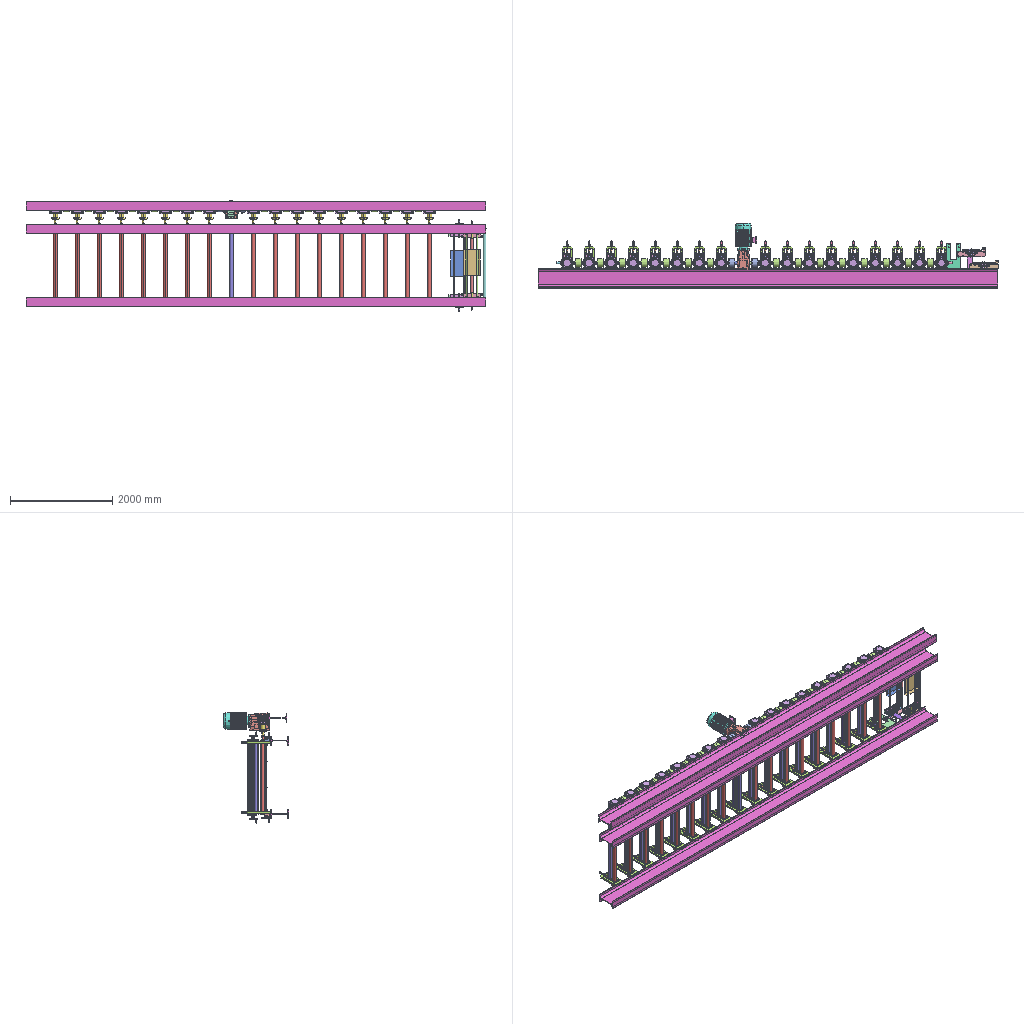Assembly | STEP file | 57 different items | 1331 placed | box 9007 x 1275 x 2167 mm
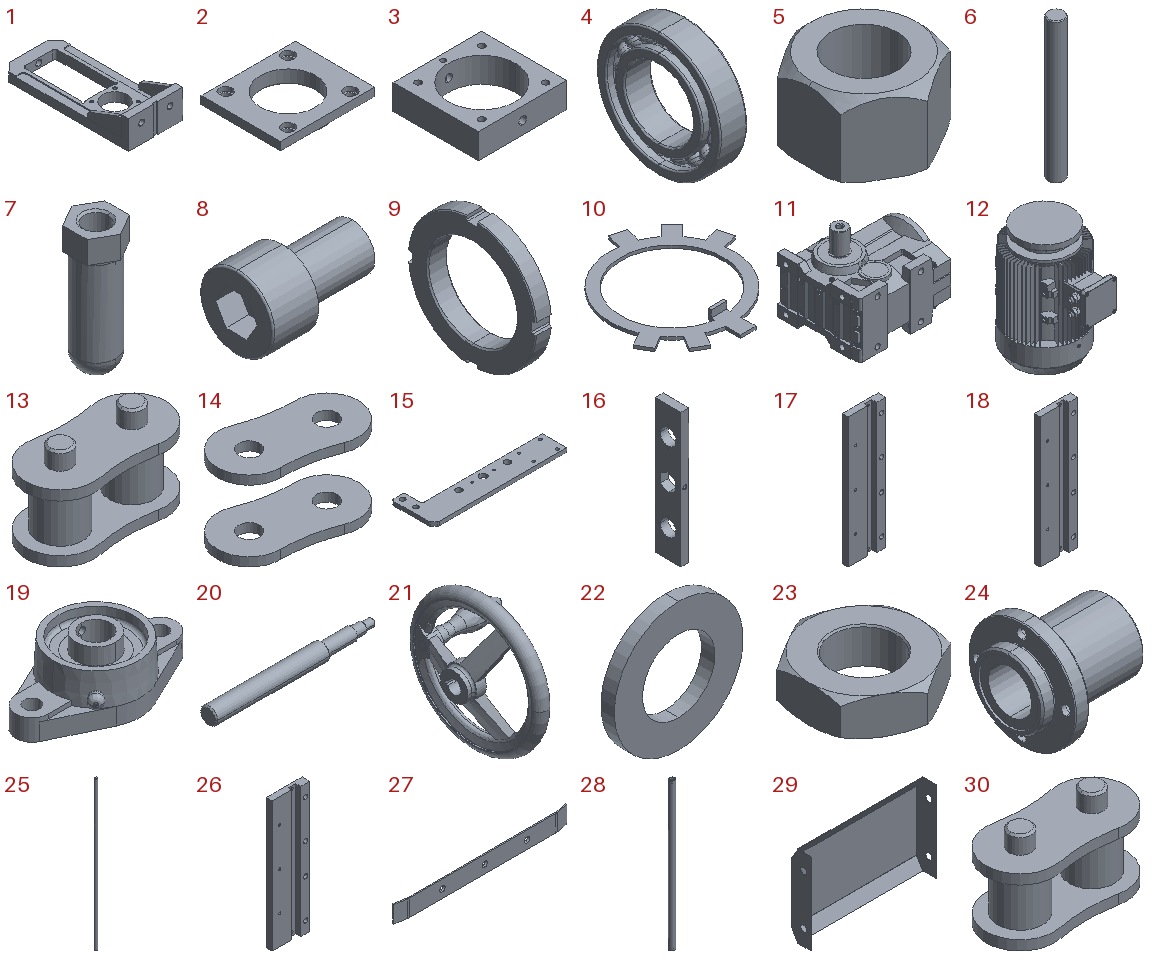Parts list (item | quantity | size | volume):
1 | x36 | 200 x 470 x 105 mm | 2366246 mm3
2 | x144 | 130 x 110 x 18 mm | 122243 mm3
3 | x36 | 120 x 115 x 34 mm | 242245 mm3
4 | x72 | 20 x 90 x 90 mm | 65276 mm3
5 | x72 | 28.536 x 32.95 x 19 mm | 8806 mm3
6 | x36 | 20 x 20 x 175 mm | 54917 mm3
7 | x36 | 30 x 34.641 x 92 mm | 50056 mm3
8 | x576 | 26 x 16 x 16 mm | 2981 mm3
9 | x72 | 11 x 69.742 x 69.742 mm | 20244 mm3
10 | x36 | 72.177 x 75.317 x 5 mm | 1971 mm3
11 | x1 | 389 x 345 x 416 mm | 22949319 mm3
12 | x1 | 323.2 x 423.482 x 518 mm | 31241978 mm3
13 | x17 | 37.13 x 18.08 x 26.9 mm | 6307 mm3
14 | x16 | 36.793 x 21.646 x 22.78 mm | 2638 mm3
15 | x2 | 549.959 x 175.002 x 16 mm | 892550 mm3
16 | x2 | 20 x 65 x 340 mm | 355958 mm3
17 | x1 | 92.98 x 19.5 x 340 mm | 429888 mm3
18 | x2 | 92.98 x 19.5 x 340 mm | 434524 mm3
19 | x2 | 113 x 62 x 37.3 mm | 69563 mm3
20 | x2 | 263 x 27 x 27 mm | 124305 mm3
21 | x2 | 117 x 160 x 160 mm | 172381 mm3
22 | x2 | 24 x 2.5 x 24 mm | 773.126 mm3
23 | x2 | 18 x 20.785 x 6 mm | 1162 mm3
24 | x4 | 59 x 62 x 62 mm | 56273 mm3
25 | x2 | 25 x 25 x 1510 mm | 741143 mm3
26 | x1 | 92.98 x 19.5 x 340 mm | 429888 mm3
27 | x4 | 409.088 x 8.069 x 40 mm | 48290 mm3
28 | x2 | 50 x 50 x 1450 mm | 1794980 mm3
29 | x1 | 504 x 80 x 327.138 mm | 217824 mm3
30 | x16 | 37.13 x 18.08 x 26.9 mm | 6307 mm3
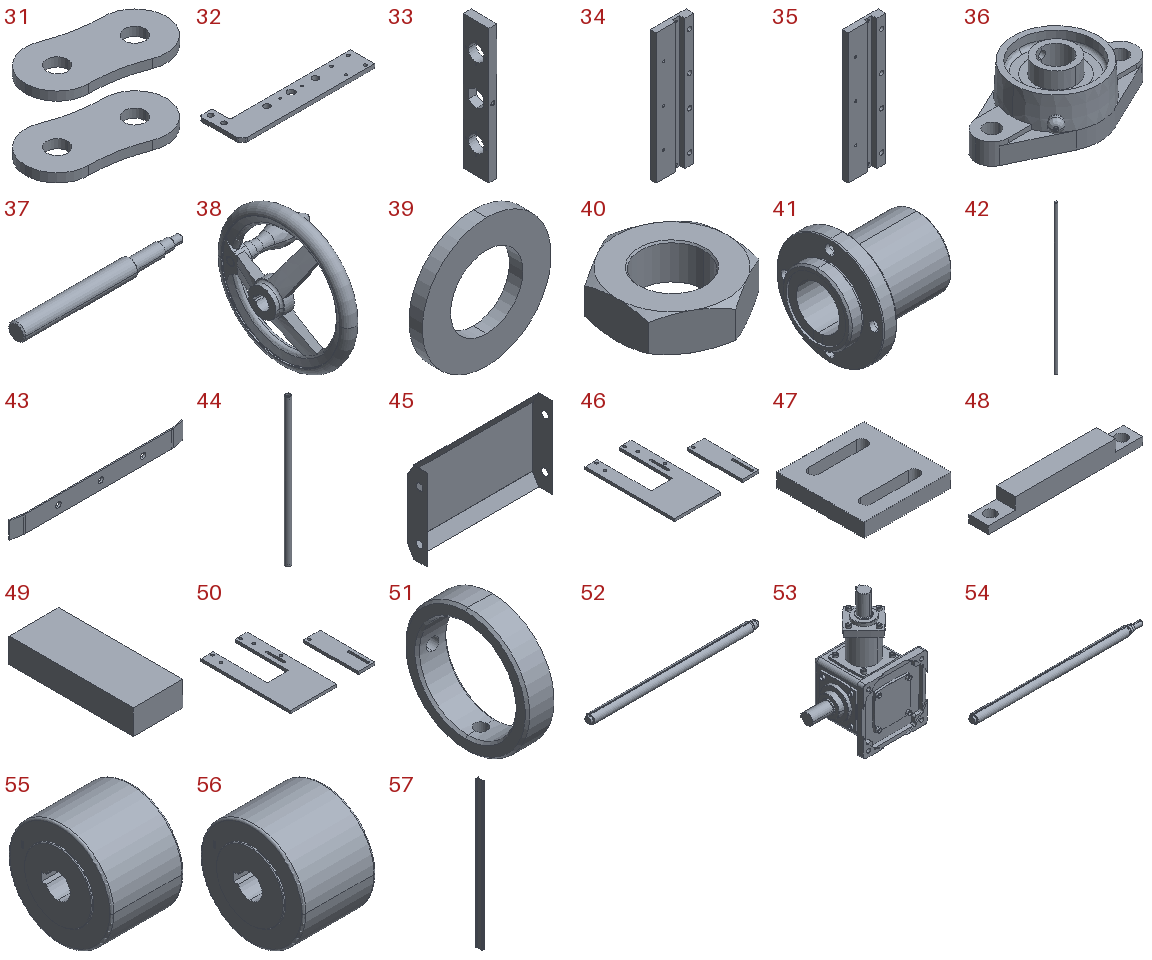31 | x16 | 36.793 x 21.646 x 22.78 mm | 2638 mm3
32 | x2 | 549.959 x 175.002 x 16 mm | 892550 mm3
33 | x2 | 20 x 65 x 340 mm | 355958 mm3
34 | x2 | 92.98 x 19.5 x 340 mm | 429888 mm3
35 | x2 | 92.98 x 19.5 x 340 mm | 434524 mm3
36 | x2 | 113 x 62 x 37.3 mm | 69563 mm3
37 | x2 | 263 x 27 x 27 mm | 124305 mm3
38 | x2 | 117 x 160 x 160 mm | 172381 mm3
39 | x2 | 24 x 2.5 x 24 mm | 773.126 mm3
40 | x2 | 18 x 20.785 x 6 mm | 1162 mm3
41 | x4 | 59 x 62 x 62 mm | 56273 mm3
42 | x2 | 25 x 25 x 1470 mm | 721508 mm3
43 | x4 | 409.088 x 8.069 x 40 mm | 48290 mm3
44 | x2 | 50 x 50 x 1410 mm | 1744715 mm3
45 | x1 | 504 x 80 x 327.138 mm | 217529 mm3
46 | x1 | 507 x 540 x 16 mm | 2169859 mm3
47 | x1 | 100 x 100 x 16 mm | 134073 mm3
48 | x1 | 200 x 25 x 25 mm | 95447 mm3
49 | x1 | 40 x 100 x 20 mm | 80000 mm3
50 | x1 | 507 x 540 x 16 mm | 2169859 mm3
51 | x8 | 8 x 32 x 32 mm | 2296 mm3
52 | x19 | 1430 x 75 x 75 mm | 6071398 mm3
53 | x17 | 416 x 229.5 x 425.5 mm | 8932434 mm3
54 | x17 | 1505 x 75 x 75 mm | 6161488 mm3
55 | x2 | 123.5 x 168 x 168 mm | 2239752 mm3
56 | x15 | 123.5 x 168 x 168 mm | 2326586 mm3
57 | x3 | 175 x 350 x 9000 mm | 85369066 mm3
Placements (level | parent | child | x y z in mm | rotation matrix by rows), first 402 of 1411 lines:
1 | subassembly 2 | subassembly 3 | 0.0 0.0 668.0 | 1 0 0 0 1 0 0 0 1
2 | subassembly 3 | subassembly 4 | -0.0 248.0 -0.0 | 1 0 0 0 1 0 0 0 1
2 | subassembly 3 | subassembly 5 | -0.0 150.0 34.0 | 1 0 0 0 1 0 0 0 1
2 | subassembly 3 | subassembly 5 | -0.0 280.0 34.0 | 1 0 0 0 1 0 0 0 1
2 | subassembly 3 | subassembly 5 | 0.0 280.0 0.0 | -1 0 0 0 1 0 0 0 -1
2 | subassembly 3 | subassembly 5 | 0.0 150.0 0.0 | -1 0 0 0 1 0 0 0 -1
2 | subassembly 3 | subassembly 6 | -0.0 282.5 -0.0 | 1 0 0 0 1 0 0 0 1
2 | subassembly 3 | subassembly 7 | -0.0 280.0 17.0 | 0 0 1 0 1 0 -1 0 0
2 | subassembly 3 | subassembly 7 | -0.0 150.0 17.0 | 0 0 1 0 1 0 -1 0 0
2 | subassembly 3 | subassembly 8 | -0.0 470.0 17.0 | 0.9291 0.3698 0 0 0 1 0.3698 -0.9291 0
2 | subassembly 3 | subassembly 8 | -0.0 411.0 17.0 | 1 0 0 0 0 1 0 -1 0
2 | subassembly 3 | subassembly 9 | -0.0 515.0 17.0 | -0.6523 0.7579 0 0 0 -1 -0.7579 -0.6523 -0
2 | subassembly 3 | subassembly 10 | -0.0 489.0 17.0 | 0.9291 -0.3698 0 0 0 -1 0.3698 0.9291 -0
2 | subassembly 3 | subassembly 11 | 42.999 107.001 -15.0 | 0 -0.4429 -0.8966 0 0.8966 -0.4429 1 0 0
2 | subassembly 3 | subassembly 11 | -42.999 107.001 -15.0 | 0 0.8966 -0.4429 0 0.4429 0.8966 1 0 0
2 | subassembly 3 | subassembly 11 | -42.999 237.001 49.0 | 0 -0.02998 -0.9996 0 -0.9996 0.02998 -1 0 0
2 | subassembly 3 | subassembly 11 | -42.999 322.999 49.0 | 0 -0.9996 0.02998 0 0.02998 0.9996 -1 0 0
2 | subassembly 3 | subassembly 11 | 42.999 192.999 -15.0 | 0 -0.8966 0.4429 0 -0.4429 -0.8966 1 0 0
2 | subassembly 3 | subassembly 11 | 42.999 237.001 -15.0 | 0 0.9996 0.02998 0 -0.02998 0.9996 1 0 0
2 | subassembly 3 | subassembly 11 | -42.999 192.999 -15.0 | 0 0.4429 0.8966 0 -0.8966 0.4429 1 0 0
2 | subassembly 3 | subassembly 11 | 42.999 237.001 49.0 | 0 0.9996 -0.02998 0 -0.02998 -0.9996 -1 0 0
2 | subassembly 3 | subassembly 11 | -42.999 192.999 49.0 | 0 0.4429 -0.8966 0 -0.8966 -0.4429 -1 0 0
2 | subassembly 3 | subassembly 11 | -42.999 322.999 -15.0 | 0 -0.9996 -0.02998 0 0.02998 -0.9996 1 0 0
2 | subassembly 3 | subassembly 11 | -42.999 107.001 49.0 | 0 0.8966 0.4429 0 0.4429 -0.8966 -1 0 0
2 | subassembly 3 | subassembly 11 | 42.999 107.001 49.0 | 0 -0.4429 0.8966 0 0.8966 0.4429 -1 0 0
2 | subassembly 3 | subassembly 11 | 42.999 322.999 49.0 | 0 0.02998 0.9996 0 0.9996 -0.02998 -1 0 0
2 | subassembly 3 | subassembly 11 | 42.999 192.999 49.0 | 0 -0.8966 -0.4429 0 -0.4429 0.8966 -1 0 0
2 | subassembly 3 | subassembly 11 | 42.999 322.999 -15.0 | 0 0.02998 -0.9996 0 0.9996 0.02998 1 0 0
2 | subassembly 3 | subassembly 11 | -42.999 237.001 -15.0 | 0 -0.02998 0.9996 0 -0.9996 -0.02998 1 0 0
1 | subassembly 2 | subassembly 12 | 431.0 -0.0 668.0 | 1 0 0 0 1 0 0 0 1
2 | subassembly 12 | subassembly 4 | -0.0 248.0 -0.0 | 1 0 0 0 1 0 0 0 1
2 | subassembly 12 | subassembly 5 | -0.0 280.0 34.0 | 1 0 0 0 1 0 0 0 1
2 | subassembly 12 | subassembly 5 | 0.0 280.0 0.0 | -1 0 0 0 1 0 0 0 -1
2 | subassembly 12 | subassembly 5 | 0.0 150.0 0.0 | -1 0 0 0 1 0 0 0 -1
2 | subassembly 12 | subassembly 5 | -0.0 150.0 34.0 | 1 0 0 0 1 0 0 0 1
2 | subassembly 12 | subassembly 6 | -0.0 282.5 -0.0 | 1 0 0 0 1 0 0 0 1
2 | subassembly 12 | subassembly 7 | -0.0 280.0 17.0 | 0 0 1 0 1 0 -1 0 0
2 | subassembly 12 | subassembly 7 | -0.0 150.0 17.0 | 0 0 1 0 1 0 -1 0 0
2 | subassembly 12 | subassembly 8 | -0.0 470.0 17.0 | 0.9291 0.3698 0 0 0 1 0.3698 -0.9291 0
2 | subassembly 12 | subassembly 8 | -0.0 411.0 17.0 | 1 0 0 0 0 1 0 -1 0
2 | subassembly 12 | subassembly 9 | -0.0 515.0 17.0 | -0.6523 0.7579 0 0 0 -1 -0.7579 -0.6523 -0
2 | subassembly 12 | subassembly 10 | -0.0 489.0 17.0 | 0.9291 -0.3698 0 0 0 -1 0.3698 0.9291 -0
2 | subassembly 12 | subassembly 11 | 42.999 237.001 49.0 | 0 0.9996 -0.02998 0 -0.02998 -0.9996 -1 0 0
2 | subassembly 12 | subassembly 11 | 42.999 322.999 49.0 | 0 0.02998 0.9996 0 0.9996 -0.02998 -1 0 0
2 | subassembly 12 | subassembly 11 | -42.999 237.001 49.0 | 0 -0.02998 -0.9996 0 -0.9996 0.02998 -1 0 0
2 | subassembly 12 | subassembly 11 | -42.999 192.999 49.0 | 0 0.4429 -0.8966 0 -0.8966 -0.4429 -1 0 0
2 | subassembly 12 | subassembly 11 | -42.999 322.999 49.0 | 0 -0.9996 0.02998 0 0.02998 0.9996 -1 0 0
2 | subassembly 12 | subassembly 11 | 42.999 107.001 49.0 | 0 -0.4429 0.8966 0 0.8966 0.4429 -1 0 0
2 | subassembly 12 | subassembly 11 | 42.999 192.999 -15.0 | 0 -0.8966 0.4429 0 -0.4429 -0.8966 1 0 0
2 | subassembly 12 | subassembly 11 | 42.999 237.001 -15.0 | 0 0.9996 0.02998 0 -0.02998 0.9996 1 0 0
2 | subassembly 12 | subassembly 11 | -42.999 237.001 -15.0 | 0 -0.02998 0.9996 0 -0.9996 -0.02998 1 0 0
2 | subassembly 12 | subassembly 11 | 42.999 192.999 49.0 | 0 -0.8966 -0.4429 0 -0.4429 0.8966 -1 0 0
2 | subassembly 12 | subassembly 11 | -42.999 107.001 -15.0 | 0 0.8966 -0.4429 0 0.4429 0.8966 1 0 0
2 | subassembly 12 | subassembly 11 | -42.999 107.001 49.0 | 0 0.8966 0.4429 0 0.4429 -0.8966 -1 0 0
2 | subassembly 12 | subassembly 11 | -42.999 322.999 -15.0 | 0 -0.9996 -0.02998 0 0.02998 -0.9996 1 0 0
2 | subassembly 12 | subassembly 11 | -42.999 192.999 -15.0 | 0 0.4429 0.8966 0 -0.8966 0.4429 1 0 0
2 | subassembly 12 | subassembly 11 | 42.999 107.001 -15.0 | 0 -0.4429 -0.8966 0 0.8966 -0.4429 1 0 0
2 | subassembly 12 | subassembly 11 | 42.999 322.999 -15.0 | 0 0.02998 -0.9996 0 0.9996 0.02998 1 0 0
1 | subassembly 2 | subassembly 13 | 862.0 -0.0 668.0 | 1 0 0 0 1 0 0 0 1
2 | subassembly 13 | subassembly 4 | -0.0 248.0 -0.0 | 1 0 0 0 1 0 0 0 1
2 | subassembly 13 | subassembly 5 | 0.0 280.0 0.0 | -1 0 0 0 1 0 0 0 -1
2 | subassembly 13 | subassembly 5 | -0.0 280.0 34.0 | 1 0 0 0 1 0 0 0 1
2 | subassembly 13 | subassembly 5 | -0.0 150.0 34.0 | 1 0 0 0 1 0 0 0 1
2 | subassembly 13 | subassembly 5 | 0.0 150.0 0.0 | -1 0 0 0 1 0 0 0 -1
2 | subassembly 13 | subassembly 6 | -0.0 282.5 -0.0 | 1 0 0 0 1 0 0 0 1
2 | subassembly 13 | subassembly 7 | -0.0 280.0 17.0 | 0 0 1 0 1 0 -1 0 0
2 | subassembly 13 | subassembly 7 | -0.0 150.0 17.0 | 0 0 1 0 1 0 -1 0 0
2 | subassembly 13 | subassembly 8 | -0.0 411.0 17.0 | 1 0 0 0 0 1 0 -1 0
2 | subassembly 13 | subassembly 8 | -0.0 470.0 17.0 | 0.9291 0.3698 0 0 0 1 0.3698 -0.9291 0
2 | subassembly 13 | subassembly 9 | -0.0 515.0 17.0 | -0.6523 0.7579 0 0 0 -1 -0.7579 -0.6523 -0
2 | subassembly 13 | subassembly 10 | -0.0 489.0 17.0 | 0.9291 -0.3698 0 0 0 -1 0.3698 0.9291 -0
2 | subassembly 13 | subassembly 11 | -42.999 237.001 49.0 | 0 -0.02998 -0.9996 0 -0.9996 0.02998 -1 0 0
2 | subassembly 13 | subassembly 11 | 42.999 322.999 49.0 | 0 0.02998 0.9996 0 0.9996 -0.02998 -1 0 0
2 | subassembly 13 | subassembly 11 | -42.999 107.001 49.0 | 0 0.8966 0.4429 0 0.4429 -0.8966 -1 0 0
2 | subassembly 13 | subassembly 11 | -42.999 322.999 -15.0 | 0 -0.9996 -0.02998 0 0.02998 -0.9996 1 0 0
2 | subassembly 13 | subassembly 11 | 42.999 237.001 49.0 | 0 0.9996 -0.02998 0 -0.02998 -0.9996 -1 0 0
2 | subassembly 13 | subassembly 11 | 42.999 322.999 -15.0 | 0 0.02998 -0.9996 0 0.9996 0.02998 1 0 0
2 | subassembly 13 | subassembly 11 | -42.999 192.999 -15.0 | 0 0.4429 0.8966 0 -0.8966 0.4429 1 0 0
2 | subassembly 13 | subassembly 11 | -42.999 237.001 -15.0 | 0 -0.02998 0.9996 0 -0.9996 -0.02998 1 0 0
2 | subassembly 13 | subassembly 11 | -42.999 322.999 49.0 | 0 -0.9996 0.02998 0 0.02998 0.9996 -1 0 0
2 | subassembly 13 | subassembly 11 | -42.999 192.999 49.0 | 0 0.4429 -0.8966 0 -0.8966 -0.4429 -1 0 0
2 | subassembly 13 | subassembly 11 | 42.999 107.001 49.0 | 0 -0.4429 0.8966 0 0.8966 0.4429 -1 0 0
2 | subassembly 13 | subassembly 11 | 42.999 192.999 49.0 | 0 -0.8966 -0.4429 0 -0.4429 0.8966 -1 0 0
2 | subassembly 13 | subassembly 11 | 42.999 237.001 -15.0 | 0 0.9996 0.02998 0 -0.02998 0.9996 1 0 0
2 | subassembly 13 | subassembly 11 | 42.999 107.001 -15.0 | 0 -0.4429 -0.8966 0 0.8966 -0.4429 1 0 0
2 | subassembly 13 | subassembly 11 | -42.999 107.001 -15.0 | 0 0.8966 -0.4429 0 0.4429 0.8966 1 0 0
2 | subassembly 13 | subassembly 11 | 42.999 192.999 -15.0 | 0 -0.8966 0.4429 0 -0.4429 -0.8966 1 0 0
1 | subassembly 2 | subassembly 14 | 1293.0 -0.0 668.0 | 1 0 0 0 1 0 0 0 1
2 | subassembly 14 | subassembly 4 | -0.0 248.0 -0.0 | 1 0 0 0 1 0 0 0 1
2 | subassembly 14 | subassembly 5 | -0.0 280.0 0.0 | -1 0 0 0 1 0 0 0 -1
2 | subassembly 14 | subassembly 5 | 0.0 150.0 0.0 | -1 0 0 0 1 0 0 0 -1
2 | subassembly 14 | subassembly 5 | -0.0 150.0 34.0 | 1 0 0 0 1 0 0 0 1
2 | subassembly 14 | subassembly 5 | -0.0 280.0 34.0 | 1 0 0 0 1 0 0 0 1
2 | subassembly 14 | subassembly 6 | -0.0 282.5 -0.0 | 1 0 0 0 1 0 0 0 1
2 | subassembly 14 | subassembly 7 | -0.0 150.0 17.0 | 0 0 1 0 1 0 -1 0 0
2 | subassembly 14 | subassembly 7 | -0.0 280.0 17.0 | 0 0 1 0 1 0 -1 0 0
2 | subassembly 14 | subassembly 8 | -0.0 470.0 17.0 | 0.9291 0.3698 0 0 0 1 0.3698 -0.9291 0
2 | subassembly 14 | subassembly 8 | -0.0 411.0 17.0 | 1 0 0 0 0 1 0 -1 0
2 | subassembly 14 | subassembly 9 | 0.0 515.0 17.0 | -0.6523 0.7579 0 0 0 -1 -0.7579 -0.6523 -0
2 | subassembly 14 | subassembly 10 | 0.0 489.0 17.0 | 0.9291 -0.3698 0 0 0 -1 0.3698 0.9291 -0
2 | subassembly 14 | subassembly 11 | -42.999 192.999 49.0 | 0 0.4429 -0.8966 0 -0.8966 -0.4429 -1 0 0
2 | subassembly 14 | subassembly 11 | 42.999 237.001 -15.0 | 0 0.9996 0.02998 0 -0.02998 0.9996 1 0 0
2 | subassembly 14 | subassembly 11 | 42.999 322.999 49.0 | 0 0.02998 0.9996 0 0.9996 -0.02998 -1 0 0
2 | subassembly 14 | subassembly 11 | 42.999 107.001 -15.0 | 0 -0.4429 -0.8966 0 0.8966 -0.4429 1 0 0
2 | subassembly 14 | subassembly 11 | -42.999 107.001 49.0 | 0 0.8966 0.4429 0 0.4429 -0.8966 -1 0 0
2 | subassembly 14 | subassembly 11 | 42.999 322.999 -15.0 | 0 0.02998 -0.9996 0 0.9996 0.02998 1 0 0
2 | subassembly 14 | subassembly 11 | -42.999 322.999 -15.0 | 0 -0.9996 -0.02998 0 0.02998 -0.9996 1 0 0
2 | subassembly 14 | subassembly 11 | -42.999 192.999 -15.0 | 0 0.4429 0.8966 0 -0.8966 0.4429 1 0 0
2 | subassembly 14 | subassembly 11 | 42.999 237.001 49.0 | 0 0.9996 -0.02998 0 -0.02998 -0.9996 -1 0 0
2 | subassembly 14 | subassembly 11 | 42.999 192.999 49.0 | 0 -0.8966 -0.4429 0 -0.4429 0.8966 -1 0 0
2 | subassembly 14 | subassembly 11 | -42.999 237.001 -15.0 | 0 -0.02998 0.9996 0 -0.9996 -0.02998 1 0 0
2 | subassembly 14 | subassembly 11 | -42.999 237.001 49.0 | 0 -0.02998 -0.9996 0 -0.9996 0.02998 -1 0 0
2 | subassembly 14 | subassembly 11 | 42.999 107.001 49.0 | 0 -0.4429 0.8966 0 0.8966 0.4429 -1 0 0
2 | subassembly 14 | subassembly 11 | 42.999 192.999 -15.0 | 0 -0.8966 0.4429 0 -0.4429 -0.8966 1 0 0
2 | subassembly 14 | subassembly 11 | -42.999 107.001 -15.0 | 0 0.8966 -0.4429 0 0.4429 0.8966 1 0 0
2 | subassembly 14 | subassembly 11 | -42.999 322.999 49.0 | 0 -0.9996 0.02998 0 0.02998 0.9996 -1 0 0
1 | subassembly 2 | subassembly 15 | 1724.0 -0.0 668.0 | 1 0 0 0 1 0 0 0 1
2 | subassembly 15 | subassembly 4 | -0.0 248.0 -0.0 | 1 0 0 0 1 0 0 0 1
2 | subassembly 15 | subassembly 5 | -0.0 280.0 34.0 | 1 0 0 0 1 0 0 0 1
2 | subassembly 15 | subassembly 5 | 0.0 150.0 0.0 | -1 0 0 0 1 0 0 0 -1
2 | subassembly 15 | subassembly 5 | -0.0 280.0 0.0 | -1 0 0 0 1 0 0 0 -1
2 | subassembly 15 | subassembly 5 | -0.0 150.0 34.0 | 1 0 0 0 1 0 0 0 1
2 | subassembly 15 | subassembly 6 | -0.0 282.5 -0.0 | 1 0 0 0 1 0 0 0 1
2 | subassembly 15 | subassembly 7 | -0.0 280.0 17.0 | 0 0 1 0 1 0 -1 0 0
2 | subassembly 15 | subassembly 7 | -0.0 150.0 17.0 | 0 0 1 0 1 0 -1 0 0
2 | subassembly 15 | subassembly 8 | -0.0 470.0 17.0 | 0.9291 0.3698 0 0 0 1 0.3698 -0.9291 0
2 | subassembly 15 | subassembly 8 | -0.0 411.0 17.0 | 1 0 0 0 0 1 0 -1 0
2 | subassembly 15 | subassembly 9 | 0.0 515.0 17.0 | -0.6523 0.7579 0 0 0 -1 -0.7579 -0.6523 -0
2 | subassembly 15 | subassembly 10 | 0.0 489.0 17.0 | 0.9291 -0.3698 0 0 0 -1 0.3698 0.9291 -0
2 | subassembly 15 | subassembly 11 | 42.999 237.001 49.0 | 0 0.9996 -0.02998 0 -0.02998 -0.9996 -1 0 0
2 | subassembly 15 | subassembly 11 | 42.999 192.999 49.0 | 0 -0.8966 -0.4429 0 -0.4429 0.8966 -1 0 0
2 | subassembly 15 | subassembly 11 | 42.999 107.001 49.0 | 0 -0.4429 0.8966 0 0.8966 0.4429 -1 0 0
2 | subassembly 15 | subassembly 11 | 42.999 322.999 49.0 | 0 0.02998 0.9996 0 0.9996 -0.02998 -1 0 0
2 | subassembly 15 | subassembly 11 | 42.999 322.999 -15.0 | 0 0.02998 -0.9996 0 0.9996 0.02998 1 0 0
2 | subassembly 15 | subassembly 11 | 42.999 237.001 -15.0 | 0 0.9996 0.02998 0 -0.02998 0.9996 1 0 0
2 | subassembly 15 | subassembly 11 | 42.999 107.001 -15.0 | 0 -0.4429 -0.8966 0 0.8966 -0.4429 1 0 0
2 | subassembly 15 | subassembly 11 | -42.999 107.001 -15.0 | 0 0.8966 -0.4429 0 0.4429 0.8966 1 0 0
2 | subassembly 15 | subassembly 11 | -42.999 237.001 -15.0 | 0 -0.02998 0.9996 0 -0.9996 -0.02998 1 0 0
2 | subassembly 15 | subassembly 11 | -42.999 237.001 49.0 | 0 -0.02998 -0.9996 0 -0.9996 0.02998 -1 0 0
2 | subassembly 15 | subassembly 11 | 42.999 192.999 -15.0 | 0 -0.8966 0.4429 0 -0.4429 -0.8966 1 0 0
2 | subassembly 15 | subassembly 11 | -42.999 322.999 49.0 | 0 -0.9996 0.02998 0 0.02998 0.9996 -1 0 0
2 | subassembly 15 | subassembly 11 | -42.999 107.001 49.0 | 0 0.8966 0.4429 0 0.4429 -0.8966 -1 0 0
2 | subassembly 15 | subassembly 11 | -42.999 322.999 -15.0 | 0 -0.9996 -0.02998 0 0.02998 -0.9996 1 0 0
2 | subassembly 15 | subassembly 11 | -42.999 192.999 49.0 | 0 0.4429 -0.8966 0 -0.8966 -0.4429 -1 0 0
2 | subassembly 15 | subassembly 11 | -42.999 192.999 -15.0 | 0 0.4429 0.8966 0 -0.8966 0.4429 1 0 0
1 | subassembly 2 | subassembly 16 | 2155.0 -0.0 668.0 | 1 0 0 0 1 0 0 0 1
2 | subassembly 16 | subassembly 4 | -0.0 248.0 -0.0 | 1 0 0 0 1 0 0 0 1
2 | subassembly 16 | subassembly 5 | -0.0 150.0 34.0 | 1 0 0 0 1 0 0 0 1
2 | subassembly 16 | subassembly 5 | 0.0 150.0 0.0 | -1 0 0 0 1 0 0 0 -1
2 | subassembly 16 | subassembly 5 | -0.0 280.0 0.0 | -1 0 0 0 1 0 0 0 -1
2 | subassembly 16 | subassembly 5 | -0.0 280.0 34.0 | 1 0 0 0 1 0 0 0 1
2 | subassembly 16 | subassembly 6 | -0.0 282.5 -0.0 | 1 0 0 0 1 0 0 0 1
2 | subassembly 16 | subassembly 7 | -0.0 280.0 17.0 | 0 0 1 0 1 0 -1 0 0
2 | subassembly 16 | subassembly 7 | -0.0 150.0 17.0 | 0 0 1 0 1 0 -1 0 0
2 | subassembly 16 | subassembly 8 | -0.0 470.0 17.0 | 0.9291 0.3698 0 0 0 1 0.3698 -0.9291 0
2 | subassembly 16 | subassembly 8 | -0.0 411.0 17.0 | 1 0 0 0 0 1 0 -1 0
2 | subassembly 16 | subassembly 9 | 0.0 515.0 17.0 | -0.6523 0.7579 0 0 0 -1 -0.7579 -0.6523 -0
2 | subassembly 16 | subassembly 10 | 0.0 489.0 17.0 | 0.9291 -0.3698 0 0 0 -1 0.3698 0.9291 -0
2 | subassembly 16 | subassembly 11 | 42.999 237.001 -15.0 | 0 0.9996 0.02998 0 -0.02998 0.9996 1 0 0
2 | subassembly 16 | subassembly 11 | -42.999 237.001 -15.0 | 0 -0.02998 0.9996 0 -0.9996 -0.02998 1 0 0
2 | subassembly 16 | subassembly 11 | -42.999 237.001 49.0 | 0 -0.02998 -0.9996 0 -0.9996 0.02998 -1 0 0
2 | subassembly 16 | subassembly 11 | -42.999 192.999 49.0 | 0 0.4429 -0.8966 0 -0.8966 -0.4429 -1 0 0
2 | subassembly 16 | subassembly 11 | 42.999 192.999 49.0 | 0 -0.8966 -0.4429 0 -0.4429 0.8966 -1 0 0
2 | subassembly 16 | subassembly 11 | -42.999 192.999 -15.0 | 0 0.4429 0.8966 0 -0.8966 0.4429 1 0 0
2 | subassembly 16 | subassembly 11 | -42.999 107.001 49.0 | 0 0.8966 0.4429 0 0.4429 -0.8966 -1 0 0
2 | subassembly 16 | subassembly 11 | 42.999 107.001 49.0 | 0 -0.4429 0.8966 0 0.8966 0.4429 -1 0 0
2 | subassembly 16 | subassembly 11 | -42.999 107.001 -15.0 | 0 0.8966 -0.4429 0 0.4429 0.8966 1 0 0
2 | subassembly 16 | subassembly 11 | 42.999 107.001 -15.0 | 0 -0.4429 -0.8966 0 0.8966 -0.4429 1 0 0
2 | subassembly 16 | subassembly 11 | 42.999 192.999 -15.0 | 0 -0.8966 0.4429 0 -0.4429 -0.8966 1 0 0
2 | subassembly 16 | subassembly 11 | -42.999 322.999 49.0 | 0 -0.9996 0.02998 0 0.02998 0.9996 -1 0 0
2 | subassembly 16 | subassembly 11 | 42.999 237.001 49.0 | 0 0.9996 -0.02998 0 -0.02998 -0.9996 -1 0 0
2 | subassembly 16 | subassembly 11 | -42.999 322.999 -15.0 | 0 -0.9996 -0.02998 0 0.02998 -0.9996 1 0 0
2 | subassembly 16 | subassembly 11 | 42.999 322.999 49.0 | 0 0.02998 0.9996 0 0.9996 -0.02998 -1 0 0
2 | subassembly 16 | subassembly 11 | 42.999 322.999 -15.0 | 0 0.02998 -0.9996 0 0.9996 0.02998 1 0 0
1 | subassembly 2 | subassembly 17 | 2586.0 -0.0 668.0 | 1 0 0 0 1 0 0 0 1
2 | subassembly 17 | subassembly 4 | -0.0 248.0 -0.0 | 1 0 0 0 1 0 0 0 1
2 | subassembly 17 | subassembly 5 | -0.0 280.0 34.0 | 1 0 0 0 1 0 0 0 1
2 | subassembly 17 | subassembly 5 | -0.0 150.0 34.0 | 1 0 0 0 1 0 0 0 1
2 | subassembly 17 | subassembly 5 | -0.0 280.0 0.0 | -1 0 0 0 1 0 0 0 -1
2 | subassembly 17 | subassembly 5 | 0.0 150.0 0.0 | -1 0 0 0 1 0 0 0 -1
2 | subassembly 17 | subassembly 6 | -0.0 282.5 -0.0 | 1 0 0 0 1 0 0 0 1
2 | subassembly 17 | subassembly 7 | -0.0 150.0 17.0 | 0 0 1 0 1 0 -1 0 0
2 | subassembly 17 | subassembly 7 | -0.0 280.0 17.0 | 0 0 1 0 1 0 -1 0 0
2 | subassembly 17 | subassembly 8 | -0.0 411.0 17.0 | 1 0 0 0 0 1 0 -1 0
2 | subassembly 17 | subassembly 8 | -0.0 470.0 17.0 | 0.9291 0.3698 0 0 0 1 0.3698 -0.9291 0
2 | subassembly 17 | subassembly 9 | 0.0 515.0 17.0 | -0.6523 0.7579 0 0 0 -1 -0.7579 -0.6523 -0
2 | subassembly 17 | subassembly 10 | 0.0 489.0 17.0 | 0.9291 -0.3698 0 0 0 -1 0.3698 0.9291 -0
2 | subassembly 17 | subassembly 11 | 42.999 107.001 49.0 | 0 -0.4429 0.8966 0 0.8966 0.4429 -1 0 0
2 | subassembly 17 | subassembly 11 | -42.999 237.001 49.0 | 0 -0.02998 -0.9996 0 -0.9996 0.02998 -1 0 0
2 | subassembly 17 | subassembly 11 | 42.999 237.001 49.0 | 0 0.9996 -0.02998 0 -0.02998 -0.9996 -1 0 0
2 | subassembly 17 | subassembly 11 | -42.999 237.001 -15.0 | 0 -0.02998 0.9996 0 -0.9996 -0.02998 1 0 0
2 | subassembly 17 | subassembly 11 | -42.999 107.001 -15.0 | 0 0.8966 -0.4429 0 0.4429 0.8966 1 0 0
2 | subassembly 17 | subassembly 11 | -42.999 322.999 -15.0 | 0 -0.9996 -0.02998 0 0.02998 -0.9996 1 0 0
2 | subassembly 17 | subassembly 11 | -42.999 192.999 49.0 | 0 0.4429 -0.8966 0 -0.8966 -0.4429 -1 0 0
2 | subassembly 17 | subassembly 11 | 42.999 192.999 -15.0 | 0 -0.8966 0.4429 0 -0.4429 -0.8966 1 0 0
2 | subassembly 17 | subassembly 11 | -42.999 322.999 49.0 | 0 -0.9996 0.02998 0 0.02998 0.9996 -1 0 0
2 | subassembly 17 | subassembly 11 | 42.999 192.999 49.0 | 0 -0.8966 -0.4429 0 -0.4429 0.8966 -1 0 0
2 | subassembly 17 | subassembly 11 | 42.999 237.001 -15.0 | 0 0.9996 0.02998 0 -0.02998 0.9996 1 0 0
2 | subassembly 17 | subassembly 11 | 42.999 322.999 -15.0 | 0 0.02998 -0.9996 0 0.9996 0.02998 1 0 0
2 | subassembly 17 | subassembly 11 | -42.999 192.999 -15.0 | 0 0.4429 0.8966 0 -0.8966 0.4429 1 0 0
2 | subassembly 17 | subassembly 11 | -42.999 107.001 49.0 | 0 0.8966 0.4429 0 0.4429 -0.8966 -1 0 0
2 | subassembly 17 | subassembly 11 | 42.999 107.001 -15.0 | 0 -0.4429 -0.8966 0 0.8966 -0.4429 1 0 0
2 | subassembly 17 | subassembly 11 | 42.999 322.999 49.0 | 0 0.02998 0.9996 0 0.9996 -0.02998 -1 0 0
1 | subassembly 2 | subassembly 18 | 3017.0 -0.0 668.0 | 1 0 0 0 1 0 0 0 1
2 | subassembly 18 | subassembly 4 | -0.0 248.0 -0.0 | 1 0 0 0 1 0 0 0 1
2 | subassembly 18 | subassembly 5 | -0.0 280.0 34.0 | 1 0 0 0 1 0 0 0 1
2 | subassembly 18 | subassembly 5 | -0.0 150.0 34.0 | 1 0 0 0 1 0 0 0 1
2 | subassembly 18 | subassembly 5 | -0.0 280.0 0.0 | -1 0 0 0 1 0 0 0 -1
2 | subassembly 18 | subassembly 5 | 0.0 150.0 0.0 | -1 0 0 0 1 0 0 0 -1
2 | subassembly 18 | subassembly 6 | -0.0 282.5 -0.0 | 1 0 0 0 1 0 0 0 1
2 | subassembly 18 | subassembly 7 | -0.0 150.0 17.0 | 0 0 1 0 1 0 -1 0 0
2 | subassembly 18 | subassembly 7 | -0.0 280.0 17.0 | 0 0 1 0 1 0 -1 0 0
2 | subassembly 18 | subassembly 8 | -0.0 411.0 17.0 | 1 0 0 0 0 1 0 -1 0
2 | subassembly 18 | subassembly 8 | -0.0 470.0 17.0 | 0.9291 0.3698 0 0 0 1 0.3698 -0.9291 0
2 | subassembly 18 | subassembly 9 | 0.0 515.0 17.0 | -0.6523 0.7579 0 0 0 -1 -0.7579 -0.6523 -0
2 | subassembly 18 | subassembly 10 | 0.0 489.0 17.0 | 0.9291 -0.3698 0 0 0 -1 0.3698 0.9291 -0
2 | subassembly 18 | subassembly 11 | -42.999 192.999 49.0 | 0 0.4429 -0.8966 0 -0.8966 -0.4429 -1 0 0
2 | subassembly 18 | subassembly 11 | -42.999 192.999 -15.0 | 0 0.4429 0.8966 0 -0.8966 0.4429 1 0 0
2 | subassembly 18 | subassembly 11 | 42.999 107.001 -15.0 | 0 -0.4429 -0.8966 0 0.8966 -0.4429 1 0 0
2 | subassembly 18 | subassembly 11 | 42.999 237.001 49.0 | 0 0.9996 -0.02998 0 -0.02998 -0.9996 -1 0 0
2 | subassembly 18 | subassembly 11 | -42.999 322.999 49.0 | 0 -0.9996 0.02998 0 0.02998 0.9996 -1 0 0
2 | subassembly 18 | subassembly 11 | -42.999 107.001 -15.0 | 0 0.8966 -0.4429 0 0.4429 0.8966 1 0 0
2 | subassembly 18 | subassembly 11 | 42.999 322.999 49.0 | 0 0.02998 0.9996 0 0.9996 -0.02998 -1 0 0
2 | subassembly 18 | subassembly 11 | -42.999 107.001 49.0 | 0 0.8966 0.4429 0 0.4429 -0.8966 -1 0 0
2 | subassembly 18 | subassembly 11 | -42.999 322.999 -15.0 | 0 -0.9996 -0.02998 0 0.02998 -0.9996 1 0 0
2 | subassembly 18 | subassembly 11 | 42.999 107.001 49.0 | 0 -0.4429 0.8966 0 0.8966 0.4429 -1 0 0
2 | subassembly 18 | subassembly 11 | 42.999 192.999 -15.0 | 0 -0.8966 0.4429 0 -0.4429 -0.8966 1 0 0
2 | subassembly 18 | subassembly 11 | 42.999 322.999 -15.0 | 0 0.02998 -0.9996 0 0.9996 0.02998 1 0 0
2 | subassembly 18 | subassembly 11 | 42.999 237.001 -15.0 | 0 0.9996 0.02998 0 -0.02998 0.9996 1 0 0
2 | subassembly 18 | subassembly 11 | -42.999 237.001 -15.0 | 0 -0.02998 0.9996 0 -0.9996 -0.02998 1 0 0
2 | subassembly 18 | subassembly 11 | 42.999 192.999 49.0 | 0 -0.8966 -0.4429 0 -0.4429 0.8966 -1 0 0
2 | subassembly 18 | subassembly 11 | -42.999 237.001 49.0 | 0 -0.02998 -0.9996 0 -0.9996 0.02998 -1 0 0
1 | subassembly 2 | subassembly 19 | 3448.0 -0.0 668.0 | 1 0 0 0 1 0 0 0 1
2 | subassembly 19 | subassembly 4 | -0.0 248.0 -0.0 | 1 0 0 0 1 0 0 0 1
2 | subassembly 19 | subassembly 5 | -0.0 280.0 34.0 | 1 0 0 0 1 0 0 0 1
2 | subassembly 19 | subassembly 5 | 0.0 150.0 0.0 | -1 0 0 0 1 0 0 0 -1
2 | subassembly 19 | subassembly 5 | -0.0 150.0 34.0 | 1 0 0 0 1 0 0 0 1
2 | subassembly 19 | subassembly 5 | -0.0 280.0 0.0 | -1 0 0 0 1 0 0 0 -1
2 | subassembly 19 | subassembly 6 | -0.0 282.5 -0.0 | 1 0 0 0 1 0 0 0 1
2 | subassembly 19 | subassembly 7 | -0.0 280.0 17.0 | 0 0 1 0 1 0 -1 0 0
2 | subassembly 19 | subassembly 7 | -0.0 150.0 17.0 | 0 0 1 0 1 0 -1 0 0
2 | subassembly 19 | subassembly 8 | -0.0 411.0 17.0 | 1 0 0 0 0 1 0 -1 0
2 | subassembly 19 | subassembly 8 | -0.0 470.0 17.0 | 0.9291 0.3698 0 0 0 1 0.3698 -0.9291 0
2 | subassembly 19 | subassembly 9 | 0.0 515.0 17.0 | -0.6523 0.7579 0 0 0 -1 -0.7579 -0.6523 -0
2 | subassembly 19 | subassembly 10 | 0.0 489.0 17.0 | 0.9291 -0.3698 0 0 0 -1 0.3698 0.9291 -0
2 | subassembly 19 | subassembly 11 | -42.999 107.001 49.0 | 0 0.8966 0.4429 0 0.4429 -0.8966 -1 0 0
2 | subassembly 19 | subassembly 11 | 42.999 107.001 49.0 | 0 -0.4429 0.8966 0 0.8966 0.4429 -1 0 0
2 | subassembly 19 | subassembly 11 | -42.999 237.001 -15.0 | 0 -0.02998 0.9996 0 -0.9996 -0.02998 1 0 0
2 | subassembly 19 | subassembly 11 | -42.999 192.999 -15.0 | 0 0.4429 0.8966 0 -0.8966 0.4429 1 0 0
2 | subassembly 19 | subassembly 11 | -42.999 192.999 49.0 | 0 0.4429 -0.8966 0 -0.8966 -0.4429 -1 0 0
2 | subassembly 19 | subassembly 11 | -42.999 107.001 -15.0 | 0 0.8966 -0.4429 0 0.4429 0.8966 1 0 0
2 | subassembly 19 | subassembly 11 | -42.999 237.001 49.0 | 0 -0.02998 -0.9996 0 -0.9996 0.02998 -1 0 0
2 | subassembly 19 | subassembly 11 | 42.999 237.001 49.0 | 0 0.9996 -0.02998 0 -0.02998 -0.9996 -1 0 0
2 | subassembly 19 | subassembly 11 | -42.999 322.999 -15.0 | 0 -0.9996 -0.02998 0 0.02998 -0.9996 1 0 0
2 | subassembly 19 | subassembly 11 | 42.999 322.999 49.0 | 0 0.02998 0.9996 0 0.9996 -0.02998 -1 0 0
2 | subassembly 19 | subassembly 11 | 42.999 237.001 -15.0 | 0 0.9996 0.02998 0 -0.02998 0.9996 1 0 0
2 | subassembly 19 | subassembly 11 | 42.999 192.999 -15.0 | 0 -0.8966 0.4429 0 -0.4429 -0.8966 1 0 0
2 | subassembly 19 | subassembly 11 | 42.999 192.999 49.0 | 0 -0.8966 -0.4429 0 -0.4429 0.8966 -1 0 0
2 | subassembly 19 | subassembly 11 | 42.999 322.999 -15.0 | 0 0.02998 -0.9996 0 0.9996 0.02998 1 0 0
2 | subassembly 19 | subassembly 11 | -42.999 322.999 49.0 | 0 -0.9996 0.02998 0 0.02998 0.9996 -1 0 0
2 | subassembly 19 | subassembly 11 | 42.999 107.001 -15.0 | 0 -0.4429 -0.8966 0 0.8966 -0.4429 1 0 0
1 | subassembly 2 | subassembly 20 | 3879.0 0.0 668.0 | 1 0 0 0 1 0 0 0 1
2 | subassembly 20 | subassembly 4 | -0.0 248.0 -0.0 | 1 0 0 0 1 0 0 0 1
2 | subassembly 20 | subassembly 5 | -0.0 280.0 34.0 | 1 0 0 0 1 0 0 0 1
2 | subassembly 20 | subassembly 5 | 0.0 150.0 0.0 | -1 0 0 0 1 0 0 0 -1
2 | subassembly 20 | subassembly 5 | -0.0 280.0 0.0 | -1 0 0 0 1 0 0 0 -1
2 | subassembly 20 | subassembly 5 | -0.0 150.0 34.0 | 1 0 0 0 1 0 0 0 1
2 | subassembly 20 | subassembly 6 | -0.0 282.5 -0.0 | 1 0 0 0 1 0 0 0 1
2 | subassembly 20 | subassembly 7 | -0.0 280.0 17.0 | 0 0 1 0 1 0 -1 0 0
2 | subassembly 20 | subassembly 7 | -0.0 150.0 17.0 | 0 0 1 0 1 0 -1 0 0
2 | subassembly 20 | subassembly 8 | -0.0 470.0 17.0 | 0.9291 0.3698 0 0 0 1 0.3698 -0.9291 0
2 | subassembly 20 | subassembly 8 | -0.0 411.0 17.0 | 1 0 0 0 0 1 0 -1 0
2 | subassembly 20 | subassembly 9 | 0.0 515.0 17.0 | -0.6523 0.7579 0 0 0 -1 -0.7579 -0.6523 -0
2 | subassembly 20 | subassembly 10 | 0.0 489.0 17.0 | 0.9291 -0.3698 0 0 0 -1 0.3698 0.9291 -0
2 | subassembly 20 | subassembly 11 | 42.999 237.001 49.0 | 0 0.9996 -0.02998 0 -0.02998 -0.9996 -1 0 0
2 | subassembly 20 | subassembly 11 | -42.999 107.001 49.0 | 0 0.8966 0.4429 0 0.4429 -0.8966 -1 0 0
2 | subassembly 20 | subassembly 11 | 42.999 107.001 49.0 | 0 -0.4429 0.8966 0 0.8966 0.4429 -1 0 0
2 | subassembly 20 | subassembly 11 | 42.999 192.999 49.0 | 0 -0.8966 -0.4429 0 -0.4429 0.8966 -1 0 0
2 | subassembly 20 | subassembly 11 | -42.999 237.001 49.0 | 0 -0.02998 -0.9996 0 -0.9996 0.02998 -1 0 0
2 | subassembly 20 | subassembly 11 | -42.999 192.999 49.0 | 0 0.4429 -0.8966 0 -0.8966 -0.4429 -1 0 0
2 | subassembly 20 | subassembly 11 | -42.999 322.999 -15.0 | 0 -0.9996 -0.02998 0 0.02998 -0.9996 1 0 0
2 | subassembly 20 | subassembly 11 | 42.999 322.999 -15.0 | 0 0.02998 -0.9996 0 0.9996 0.02998 1 0 0
2 | subassembly 20 | subassembly 11 | 42.999 237.001 -15.0 | 0 0.9996 0.02998 0 -0.02998 0.9996 1 0 0
2 | subassembly 20 | subassembly 11 | -42.999 322.999 49.0 | 0 -0.9996 0.02998 0 0.02998 0.9996 -1 0 0
2 | subassembly 20 | subassembly 11 | 42.999 322.999 49.0 | 0 0.02998 0.9996 0 0.9996 -0.02998 -1 0 0
2 | subassembly 20 | subassembly 11 | -42.999 237.001 -15.0 | 0 -0.02998 0.9996 0 -0.9996 -0.02998 1 0 0
2 | subassembly 20 | subassembly 11 | -42.999 192.999 -15.0 | 0 0.4429 0.8966 0 -0.8966 0.4429 1 0 0
2 | subassembly 20 | subassembly 11 | 42.999 192.999 -15.0 | 0 -0.8966 0.4429 0 -0.4429 -0.8966 1 0 0
2 | subassembly 20 | subassembly 11 | -42.999 107.001 -15.0 | 0 0.8966 -0.4429 0 0.4429 0.8966 1 0 0
2 | subassembly 20 | subassembly 11 | 42.999 107.001 -15.0 | 0 -0.4429 -0.8966 0 0.8966 -0.4429 1 0 0
1 | subassembly 2 | subassembly 21 | 4310.0 -0.0 668.0 | 1 0 0 0 1 0 0 0 1
2 | subassembly 21 | subassembly 4 | -0.0 248.0 -0.0 | 1 0 0 0 1 0 0 0 1
2 | subassembly 21 | subassembly 5 | -0.0 280.0 0.0 | -1 0 0 0 1 0 0 0 -1
2 | subassembly 21 | subassembly 5 | -0.0 150.0 34.0 | 1 0 0 0 1 0 0 0 1
2 | subassembly 21 | subassembly 5 | 0.0 150.0 0.0 | -1 0 0 0 1 0 0 0 -1
2 | subassembly 21 | subassembly 5 | -0.0 280.0 34.0 | 1 0 0 0 1 0 0 0 1
2 | subassembly 21 | subassembly 6 | -0.0 282.5 -0.0 | 1 0 0 0 1 0 0 0 1
2 | subassembly 21 | subassembly 7 | -0.0 280.0 17.0 | 0 0 1 0 1 0 -1 0 0
2 | subassembly 21 | subassembly 7 | -0.0 150.0 17.0 | 0 0 1 0 1 0 -1 0 0
2 | subassembly 21 | subassembly 8 | -0.0 470.0 17.0 | 0.9291 0.3698 0 0 0 1 0.3698 -0.9291 0
2 | subassembly 21 | subassembly 8 | -0.0 411.0 17.0 | 1 0 0 0 0 1 0 -1 0
2 | subassembly 21 | subassembly 9 | 0.0 515.0 17.0 | -0.6523 0.7579 0 0 0 -1 -0.7579 -0.6523 -0
2 | subassembly 21 | subassembly 10 | 0.0 489.0 17.0 | 0.9291 -0.3698 0 0 0 -1 0.3698 0.9291 -0
2 | subassembly 21 | subassembly 11 | -42.999 237.001 49.0 | 0 -0.02998 -0.9996 0 -0.9996 0.02998 -1 0 0
2 | subassembly 21 | subassembly 11 | -42.999 237.001 -15.0 | 0 -0.02998 0.9996 0 -0.9996 -0.02998 1 0 0
2 | subassembly 21 | subassembly 11 | -42.999 322.999 49.0 | 0 -0.9996 0.02998 0 0.02998 0.9996 -1 0 0
2 | subassembly 21 | subassembly 11 | 42.999 237.001 49.0 | 0 0.9996 -0.02998 0 -0.02998 -0.9996 -1 0 0
2 | subassembly 21 | subassembly 11 | 42.999 322.999 49.0 | 0 0.02998 0.9996 0 0.9996 -0.02998 -1 0 0
2 | subassembly 21 | subassembly 11 | 42.999 322.999 -15.0 | 0 0.02998 -0.9996 0 0.9996 0.02998 1 0 0
2 | subassembly 21 | subassembly 11 | 42.999 192.999 -15.0 | 0 -0.8966 0.4429 0 -0.4429 -0.8966 1 0 0
2 | subassembly 21 | subassembly 11 | 42.999 237.001 -15.0 | 0 0.9996 0.02998 0 -0.02998 0.9996 1 0 0
2 | subassembly 21 | subassembly 11 | -42.999 192.999 -15.0 | 0 0.4429 0.8966 0 -0.8966 0.4429 1 0 0
2 | subassembly 21 | subassembly 11 | -42.999 192.999 49.0 | 0 0.4429 -0.8966 0 -0.8966 -0.4429 -1 0 0
2 | subassembly 21 | subassembly 11 | 42.999 107.001 49.0 | 0 -0.4429 0.8966 0 0.8966 0.4429 -1 0 0
2 | subassembly 21 | subassembly 11 | -42.999 107.001 -15.0 | 0 0.8966 -0.4429 0 0.4429 0.8966 1 0 0
2 | subassembly 21 | subassembly 11 | 42.999 192.999 49.0 | 0 -0.8966 -0.4429 0 -0.4429 0.8966 -1 0 0
2 | subassembly 21 | subassembly 11 | -42.999 322.999 -15.0 | 0 -0.9996 -0.02998 0 0.02998 -0.9996 1 0 0
2 | subassembly 21 | subassembly 11 | 42.999 107.001 -15.0 | 0 -0.4429 -0.8966 0 0.8966 -0.4429 1 0 0
2 | subassembly 21 | subassembly 11 | -42.999 107.001 49.0 | 0 0.8966 0.4429 0 0.4429 -0.8966 -1 0 0
1 | subassembly 2 | subassembly 22 | 4741.0 -0.0 668.0 | 1 0 0 0 1 0 0 0 1
2 | subassembly 22 | subassembly 4 | -0.0 248.0 -0.0 | 1 0 0 0 1 0 0 0 1
2 | subassembly 22 | subassembly 5 | -0.0 280.0 0.0 | -1 0 0 0 1 0 0 0 -1
2 | subassembly 22 | subassembly 5 | -0.0 150.0 34.0 | 1 0 0 0 1 0 0 0 1
2 | subassembly 22 | subassembly 5 | -0.0 280.0 34.0 | 1 0 0 0 1 0 0 0 1
2 | subassembly 22 | subassembly 5 | 0.0 150.0 0.0 | -1 0 0 0 1 0 0 0 -1
2 | subassembly 22 | subassembly 6 | -0.0 282.5 -0.0 | 1 0 0 0 1 0 0 0 1
2 | subassembly 22 | subassembly 7 | -0.0 280.0 17.0 | 0 0 1 0 1 0 -1 0 0
2 | subassembly 22 | subassembly 7 | -0.0 150.0 17.0 | 0 0 1 0 1 0 -1 0 0
2 | subassembly 22 | subassembly 8 | -0.0 470.0 17.0 | 0.9291 0.3698 0 0 0 1 0.3698 -0.9291 0
2 | subassembly 22 | subassembly 8 | -0.0 411.0 17.0 | 1 0 0 0 0 1 0 -1 0
2 | subassembly 22 | subassembly 9 | 0.0 515.0 17.0 | -0.6523 0.7579 0 0 0 -1 -0.7579 -0.6523 -0
2 | subassembly 22 | subassembly 10 | 0.0 489.0 17.0 | 0.9291 -0.3698 0 0 0 -1 0.3698 0.9291 -0
2 | subassembly 22 | subassembly 11 | -42.999 322.999 49.0 | 0 -0.9996 0.02998 0 0.02998 0.9996 -1 0 0
2 | subassembly 22 | subassembly 11 | 42.999 237.001 49.0 | 0 0.9996 -0.02998 0 -0.02998 -0.9996 -1 0 0
2 | subassembly 22 | subassembly 11 | 42.999 107.001 49.0 | 0 -0.4429 0.8966 0 0.8966 0.4429 -1 0 0
2 | subassembly 22 | subassembly 11 | -42.999 237.001 -15.0 | 0 -0.02998 0.9996 0 -0.9996 -0.02998 1 0 0
2 | subassembly 22 | subassembly 11 | -42.999 192.999 -15.0 | 0 0.4429 0.8966 0 -0.8966 0.4429 1 0 0
2 | subassembly 22 | subassembly 11 | 42.999 192.999 49.0 | 0 -0.8966 -0.4429 0 -0.4429 0.8966 -1 0 0
2 | subassembly 22 | subassembly 11 | -42.999 107.001 49.0 | 0 0.8966 0.4429 0 0.4429 -0.8966 -1 0 0
2 | subassembly 22 | subassembly 11 | -42.999 322.999 -15.0 | 0 -0.9996 -0.02998 0 0.02998 -0.9996 1 0 0
2 | subassembly 22 | subassembly 11 | 42.999 322.999 49.0 | 0 0.02998 0.9996 0 0.9996 -0.02998 -1 0 0
2 | subassembly 22 | subassembly 11 | 42.999 237.001 -15.0 | 0 0.9996 0.02998 0 -0.02998 0.9996 1 0 0
2 | subassembly 22 | subassembly 11 | 42.999 192.999 -15.0 | 0 -0.8966 0.4429 0 -0.4429 -0.8966 1 0 0
2 | subassembly 22 | subassembly 11 | 42.999 107.001 -15.0 | 0 -0.4429 -0.8966 0 0.8966 -0.4429 1 0 0
2 | subassembly 22 | subassembly 11 | -42.999 192.999 49.0 | 0 0.4429 -0.8966 0 -0.8966 -0.4429 -1 0 0
2 | subassembly 22 | subassembly 11 | 42.999 322.999 -15.0 | 0 0.02998 -0.9996 0 0.9996 0.02998 1 0 0
2 | subassembly 22 | subassembly 11 | -42.999 237.001 49.0 | 0 -0.02998 -0.9996 0 -0.9996 0.02998 -1 0 0
2 | subassembly 22 | subassembly 11 | -42.999 107.001 -15.0 | 0 0.8966 -0.4429 0 0.4429 0.8966 1 0 0
1 | subassembly 2 | subassembly 23 | 5172.0 -0.0 668.0 | 1 0 0 0 1 0 0 0 1
2 | subassembly 23 | subassembly 4 | -0.0 248.0 -0.0 | 1 0 0 0 1 0 0 0 1
2 | subassembly 23 | subassembly 5 | -0.0 280.0 34.0 | 1 0 0 0 1 0 0 0 1
2 | subassembly 23 | subassembly 5 | -0.0 150.0 34.0 | 1 0 0 0 1 0 0 0 1
2 | subassembly 23 | subassembly 5 | 0.0 150.0 0.0 | -1 0 0 0 1 0 0 0 -1
2 | subassembly 23 | subassembly 5 | -0.0 280.0 0.0 | -1 0 0 0 1 0 0 0 -1
2 | subassembly 23 | subassembly 6 | -0.0 282.5 -0.0 | 1 0 0 0 1 0 0 0 1
2 | subassembly 23 | subassembly 7 | -0.0 280.0 17.0 | 0 0 1 0 1 0 -1 0 0
2 | subassembly 23 | subassembly 7 | -0.0 150.0 17.0 | 0 0 1 0 1 0 -1 0 0
2 | subassembly 23 | subassembly 8 | -0.0 411.0 17.0 | 1 0 0 0 0 1 0 -1 0
2 | subassembly 23 | subassembly 8 | -0.0 470.0 17.0 | 0.9291 0.3698 0 0 0 1 0.3698 -0.9291 0
2 | subassembly 23 | subassembly 9 | 0.0 515.0 17.0 | -0.6523 0.7579 0 0 0 -1 -0.7579 -0.6523 -0
2 | subassembly 23 | subassembly 10 | 0.0 489.0 17.0 | 0.9291 -0.3698 0 0 0 -1 0.3698 0.9291 -0
2 | subassembly 23 | subassembly 11 | 42.999 107.001 49.0 | 0 -0.4429 0.8966 0 0.8966 0.4429 -1 0 0
2 | subassembly 23 | subassembly 11 | 42.999 107.001 -15.0 | 0 -0.4429 -0.8966 0 0.8966 -0.4429 1 0 0
2 | subassembly 23 | subassembly 11 | 42.999 322.999 -15.0 | 0 0.02998 -0.9996 0 0.9996 0.02998 1 0 0
2 | subassembly 23 | subassembly 11 | -42.999 322.999 -15.0 | 0 -0.9996 -0.02998 0 0.02998 -0.9996 1 0 0
2 | subassembly 23 | subassembly 11 | 42.999 322.999 49.0 | 0 0.02998 0.9996 0 0.9996 -0.02998 -1 0 0
2 | subassembly 23 | subassembly 11 | -42.999 192.999 -15.0 | 0 0.4429 0.8966 0 -0.8966 0.4429 1 0 0
2 | subassembly 23 | subassembly 11 | -42.999 192.999 49.0 | 0 0.4429 -0.8966 0 -0.8966 -0.4429 -1 0 0
2 | subassembly 23 | subassembly 11 | -42.999 322.999 49.0 | 0 -0.9996 0.02998 0 0.02998 0.9996 -1 0 0
2 | subassembly 23 | subassembly 11 | -42.999 107.001 -15.0 | 0 0.8966 -0.4429 0 0.4429 0.8966 1 0 0
2 | subassembly 23 | subassembly 11 | -42.999 107.001 49.0 | 0 0.8966 0.4429 0 0.4429 -0.8966 -1 0 0
2 | subassembly 23 | subassembly 11 | 42.999 192.999 49.0 | 0 -0.8966 -0.4429 0 -0.4429 0.8966 -1 0 0
2 | subassembly 23 | subassembly 11 | -42.999 237.001 -15.0 | 0 -0.02998 0.9996 0 -0.9996 -0.02998 1 0 0
2 | subassembly 23 | subassembly 11 | 42.999 237.001 49.0 | 0 0.9996 -0.02998 0 -0.02998 -0.9996 -1 0 0
2 | subassembly 23 | subassembly 11 | 42.999 237.001 -15.0 | 0 0.9996 0.02998 0 -0.02998 0.9996 1 0 0
2 | subassembly 23 | subassembly 11 | 42.999 192.999 -15.0 | 0 -0.8966 0.4429 0 -0.4429 -0.8966 1 0 0
2 | subassembly 23 | subassembly 11 | -42.999 237.001 49.0 | 0 -0.02998 -0.9996 0 -0.9996 0.02998 -1 0 0
1 | subassembly 2 | subassembly 24 | 5603.0 -0.0 668.0 | 1 0 0 0 1 0 0 0 1
2 | subassembly 24 | subassembly 4 | -0.0 248.0 -0.0 | 1 0 0 0 1 0 0 0 1
2 | subassembly 24 | subassembly 5 | -0.0 150.0 34.0 | 1 0 0 0 1 0 0 0 1
2 | subassembly 24 | subassembly 5 | -0.0 280.0 34.0 | 1 0 0 0 1 0 0 0 1
2 | subassembly 24 | subassembly 5 | -0.0 280.0 0.0 | -1 0 0 0 1 0 0 0 -1
2 | subassembly 24 | subassembly 5 | 0.0 150.0 0.0 | -1 0 0 0 1 0 0 0 -1
2 | subassembly 24 | subassembly 6 | -0.0 282.5 -0.0 | 1 0 0 0 1 0 0 0 1
2 | subassembly 24 | subassembly 7 | -0.0 280.0 17.0 | 0 0 1 0 1 0 -1 0 0
2 | subassembly 24 | subassembly 7 | -0.0 150.0 17.0 | 0 0 1 0 1 0 -1 0 0
2 | subassembly 24 | subassembly 8 | -0.0 470.0 17.0 | 0.9291 0.3698 0 0 0 1 0.3698 -0.9291 0
2 | subassembly 24 | subassembly 8 | -0.0 411.0 17.0 | 1 0 0 0 0 1 0 -1 0
2 | subassembly 24 | subassembly 9 | 0.0 515.0 17.0 | -0.6523 0.7579 0 0 0 -1 -0.7579 -0.6523 -0
2 | subassembly 24 | subassembly 10 | 0.0 489.0 17.0 | 0.9291 -0.3698 0 0 0 -1 0.3698 0.9291 -0
2 | subassembly 24 | subassembly 11 | -42.999 322.999 49.0 | 0 -0.9996 0.02998 0 0.02998 0.9996 -1 0 0
2 | subassembly 24 | subassembly 11 | 42.999 192.999 49.0 | 0 -0.8966 -0.4429 0 -0.4429 0.8966 -1 0 0
2 | subassembly 24 | subassembly 11 | -42.999 107.001 -15.0 | 0 0.8966 -0.4429 0 0.4429 0.8966 1 0 0
2 | subassembly 24 | subassembly 11 | 42.999 107.001 -15.0 | 0 -0.4429 -0.8966 0 0.8966 -0.4429 1 0 0
2 | subassembly 24 | subassembly 11 | -42.999 237.001 -15.0 | 0 -0.02998 0.9996 0 -0.9996 -0.02998 1 0 0
2 | subassembly 24 | subassembly 11 | 42.999 322.999 49.0 | 0 0.02998 0.9996 0 0.9996 -0.02998 -1 0 0
2 | subassembly 24 | subassembly 11 | -42.999 107.001 49.0 | 0 0.8966 0.4429 0 0.4429 -0.8966 -1 0 0
2 | subassembly 24 | subassembly 11 | 42.999 237.001 -15.0 | 0 0.9996 0.02998 0 -0.02998 0.9996 1 0 0
2 | subassembly 24 | subassembly 11 | -42.999 237.001 49.0 | 0 -0.02998 -0.9996 0 -0.9996 0.02998 -1 0 0
2 | subassembly 24 | subassembly 11 | 42.999 237.001 49.0 | 0 0.9996 -0.02998 0 -0.02998 -0.9996 -1 0 0
2 | subassembly 24 | subassembly 11 | -42.999 192.999 49.0 | 0 0.4429 -0.8966 0 -0.8966 -0.4429 -1 0 0
2 | subassembly 24 | subassembly 11 | -42.999 322.999 -15.0 | 0 -0.9996 -0.02998 0 0.02998 -0.9996 1 0 0